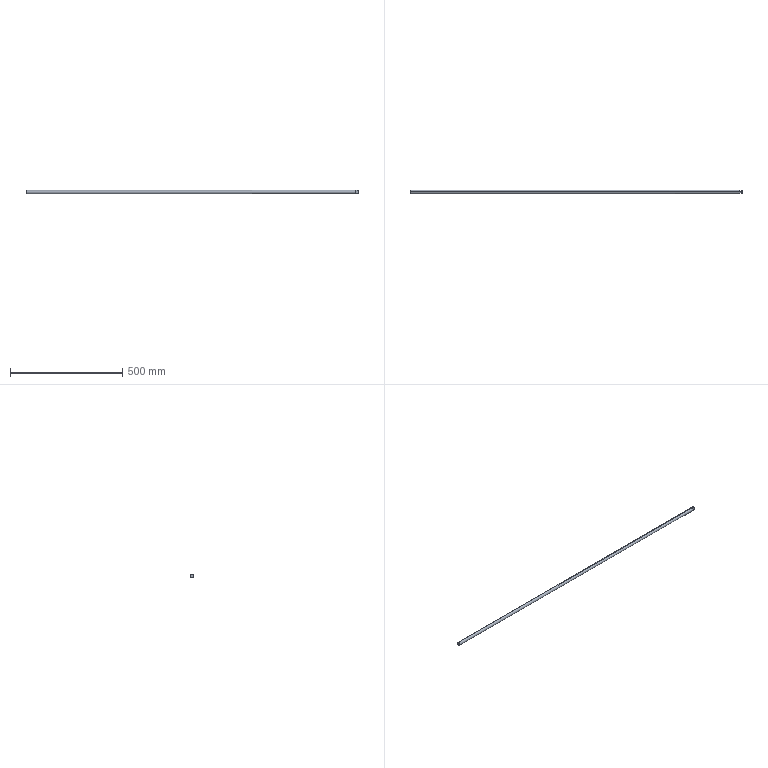Part | SolidWorks | features HoleWzd 2, Chamfer 1, Extrusion 1, ICE 1 | 1 solid | 13 faces | box 1480 x 15 x 15 mm | volume 261335 mm3 | plane 6 | cone 5 | cylinder 2 | commonest cylinder face diameters 15 x2
STEP:
#1=CARTESIAN_POINT('',(0.,0.,6.5));
#2=VERTEX_POINT('',#1);
#3=CARTESIAN_POINT('',(0.,0.,-6.5));
#4=VERTEX_POINT('',#3);
#5=CARTESIAN_POINT('',(0.,0.,0.));
#6=DIRECTION('',(-1.,0.,0.));
#7=DIRECTION('',(0.,0.,-1.));
#8=AXIS2_PLACEMENT_3D('',#5,#6,#7);
#9=CIRCLE('',#8,6.5);
#10=EDGE_CURVE('',#2,#4,#9,.T.);
#11=ORIENTED_EDGE('',*,*,#10,.F.);
#12=CARTESIAN_POINT('',(1.,0.,7.5));
#13=VERTEX_POINT('',#12);
#14=CARTESIAN_POINT('',(1.,0.,7.5));
#15=DIRECTION('',(0.7071,0.,0.7071));
#16=VECTOR('',#15,1000.);
#17=LINE('',#14,#16);
#18=EDGE_CURVE('',#2,#13,#17,.T.);
#19=ORIENTED_EDGE('',*,*,#18,.T.);
#20=CARTESIAN_POINT('',(1.,0.,-7.5));
#21=VERTEX_POINT('',#20);
#22=CARTESIAN_POINT('',(1.,0.,0.));
#23=DIRECTION('',(1.,0.,0.));
#24=DIRECTION('',(0.,0.,-1.));
#25=AXIS2_PLACEMENT_3D('',#22,#23,#24);
#26=CIRCLE('',#25,7.5);
#27=EDGE_CURVE('',#21,#13,#26,.T.);
#28=ORIENTED_EDGE('',*,*,#27,.F.);
#29=CARTESIAN_POINT('',(1.,0.,-7.5));
#30=DIRECTION('',(0.7071,0.,-0.7071));
#31=VECTOR('',#30,1000.);
#32=LINE('',#29,#31);
#33=EDGE_CURVE('',#4,#21,#32,.T.);
#34=ORIENTED_EDGE('',*,*,#33,.F.);
#35=EDGE_LOOP('',(#11,#19,#28,#34));
#36=FACE_OUTER_BOUND('',#35,.T.);
#37=CARTESIAN_POINT('',(1.,0.,0.));
#38=DIRECTION('',(1.,0.,0.));
#39=DIRECTION('',(0.,0.,-1.));
#40=AXIS2_PLACEMENT_3D('',#37,#38,#39);
#41=CONICAL_SURFACE('',#40,7.5,0.7854);
#42=ADVANCED_FACE('',(#36),#41,.T.);
#43=CARTESIAN_POINT('',(1479.,6.,-4.5));
#44=VERTEX_POINT('',#43);
#45=CARTESIAN_POINT('',(1479.,0.,-7.5));
#46=VERTEX_POINT('',#45);
#47=CARTESIAN_POINT('',(1479.,0.,0.));
#48=DIRECTION('',(-1.,0.,0.));
#49=DIRECTION('',(0.,0.,-1.));
#50=AXIS2_PLACEMENT_3D('',#47,#48,#49);
#51=CIRCLE('',#50,7.5);
#52=EDGE_CURVE('',#44,#46,#51,.T.);
#53=ORIENTED_EDGE('',*,*,#52,.T.);
#54=CARTESIAN_POINT('',(1480.,0.,-7.5));
#55=DIRECTION('',(-1.,0.,0.));
#56=VECTOR('',#55,1000.);
#57=LINE('',#54,#56);
#58=EDGE_CURVE('',#46,#21,#57,.T.);
#59=ORIENTED_EDGE('',*,*,#58,.T.);
#60=ORIENTED_EDGE('',*,*,#27,.T.);
#61=CARTESIAN_POINT('',(1479.,0.,7.5));
#62=VERTEX_POINT('',#61);
#63=CARTESIAN_POINT('',(1480.,0.,7.5));
#64=DIRECTION('',(-1.,0.,0.));
#65=VECTOR('',#64,1000.);
#66=LINE('',#63,#65);
#67=EDGE_CURVE('',#62,#13,#66,.T.);
#68=ORIENTED_EDGE('',*,*,#67,.F.);
#69=CARTESIAN_POINT('',(1479.,6.,4.5));
#70=VERTEX_POINT('',#69);
#71=CARTESIAN_POINT('',(1479.,0.,0.));
#72=DIRECTION('',(-1.,0.,0.));
#73=DIRECTION('',(0.,0.,-1.));
#74=AXIS2_PLACEMENT_3D('',#71,#72,#73);
#75=CIRCLE('',#74,7.5);
#76=EDGE_CURVE('',#62,#70,#75,.T.);
#77=ORIENTED_EDGE('',*,*,#76,.T.);
#78=CARTESIAN_POINT('',(1471.,6.,4.5));
#79=VERTEX_POINT('',#78);
#80=CARTESIAN_POINT('',(1480.,6.,4.5));
#81=DIRECTION('',(-1.,0.,0.));
#82=VECTOR('',#81,1000.);
#83=LINE('',#80,#82);
#84=EDGE_CURVE('',#70,#79,#83,.T.);
#85=ORIENTED_EDGE('',*,*,#84,.T.);
#86=CARTESIAN_POINT('',(1471.,6.,-4.5));
#87=VERTEX_POINT('',#86);
#88=CARTESIAN_POINT('',(1471.,0.,0.));
#89=DIRECTION('',(-1.,0.,0.));
#90=DIRECTION('',(0.,0.,1.));
#91=AXIS2_PLACEMENT_3D('',#88,#89,#90);
#92=CIRCLE('',#91,7.5);
#93=EDGE_CURVE('',#79,#87,#92,.T.);
#94=ORIENTED_EDGE('',*,*,#93,.T.);
#95=CARTESIAN_POINT('',(1480.,6.,-4.5));
#96=DIRECTION('',(1.,0.,0.));
#97=VECTOR('',#96,1000.);
#98=LINE('',#95,#97);
#99=EDGE_CURVE('',#87,#44,#98,.T.);
#100=ORIENTED_EDGE('',*,*,#99,.T.);
#101=EDGE_LOOP('',(#53,#59,#60,#68,#77,#85,#94,#100));
#102=FACE_OUTER_BOUND('',#101,.T.);
#103=CARTESIAN_POINT('',(1480.,0.,0.));
#104=DIRECTION('',(-1.,0.,0.));
#105=DIRECTION('',(0.,0.,1.));
#106=AXIS2_PLACEMENT_3D('',#103,#104,#105);
#107=CYLINDRICAL_SURFACE('',#106,7.5);
#108=ADVANCED_FACE('',(#102),#107,.T.);
#109=CARTESIAN_POINT('',(1480.,0.,6.5));
#110=VERTEX_POINT('',#109);
#111=CARTESIAN_POINT('',(1480.,-6.,2.5));
#112=VERTEX_POINT('',#111);
#113=CARTESIAN_POINT('',(1480.,0.,0.));
#114=DIRECTION('',(1.,0.,0.));
#115=DIRECTION('',(0.,0.,-1.));
#116=AXIS2_PLACEMENT_3D('',#113,#114,#115);
#117=CIRCLE('',#116,6.5);
#118=EDGE_CURVE('',#110,#112,#117,.T.);
#119=ORIENTED_EDGE('',*,*,#118,.F.);
#120=CARTESIAN_POINT('',(1480.,0.,6.5));
#121=DIRECTION('',(-0.7071,0.,0.7071));
#122=VECTOR('',#121,1000.);
#123=LINE('',#120,#122);
#124=EDGE_CURVE('',#110,#62,#123,.T.);
#125=ORIENTED_EDGE('',*,*,#124,.T.);
#126=CARTESIAN_POINT('',(1479.,-6.,4.5));
#127=VERTEX_POINT('',#126);
#128=CARTESIAN_POINT('',(1479.,0.,0.));
#129=DIRECTION('',(-1.,0.,0.));
#130=DIRECTION('',(0.,0.,-1.));
#131=AXIS2_PLACEMENT_3D('',#128,#129,#130);
#132=CIRCLE('',#131,7.5);
#133=EDGE_CURVE('',#127,#62,#132,.T.);
#134=ORIENTED_EDGE('',*,*,#133,.F.);
#135=CARTESIAN_POINT('',(1480.,-6.,2.5));
#136=CARTESIAN_POINT('',(1479.73,-6.,3.203));
#137=CARTESIAN_POINT('',(1479.383,-6.,3.862));
#138=CARTESIAN_POINT('',(1479.,-6.,4.5));
#139=B_SPLINE_CURVE_WITH_KNOTS('',3,(#135,#136,#137,#138),.UNSPECIFIED.,.F.,.F.,(4,4),(0.02153,0.02379),.UNSPECIFIED.);
#140=EDGE_CURVE('',#112,#127,#139,.T.);
#141=ORIENTED_EDGE('',*,*,#140,.F.);
#142=EDGE_LOOP('',(#119,#125,#134,#141));
#143=FACE_OUTER_BOUND('',#142,.T.);
#144=CARTESIAN_POINT('',(1480.,0.,0.));
#145=DIRECTION('',(-1.,0.,0.));
#146=DIRECTION('',(0.,0.,1.));
#147=AXIS2_PLACEMENT_3D('',#144,#145,#146);
#148=CONICAL_SURFACE('',#147,6.5,0.7854);
#149=ADVANCED_FACE('',(#143),#148,.T.);
#150=ORIENTED_EDGE('',*,*,#124,.F.);
#151=CARTESIAN_POINT('',(1480.,6.,2.5));
#152=VERTEX_POINT('',#151);
#153=CARTESIAN_POINT('',(1480.,0.,0.));
#154=DIRECTION('',(1.,0.,0.));
#155=DIRECTION('',(0.,0.,-1.));
#156=AXIS2_PLACEMENT_3D('',#153,#154,#155);
#157=CIRCLE('',#156,6.5);
#158=EDGE_CURVE('',#152,#110,#157,.T.);
#159=ORIENTED_EDGE('',*,*,#158,.F.);
#160=CARTESIAN_POINT('',(1479.,6.,4.5));
#161=CARTESIAN_POINT('',(1479.385,6.,3.859));
#162=CARTESIAN_POINT('',(1479.731,6.,3.198));
#163=CARTESIAN_POINT('',(1480.,6.,2.5));
#164=B_SPLINE_CURVE_WITH_KNOTS('',3,(#160,#161,#162,#163),.UNSPECIFIED.,.F.,.F.,(4,4),(0.01416,0.0164),.UNSPECIFIED.);
#165=EDGE_CURVE('',#70,#152,#164,.T.);
#166=ORIENTED_EDGE('',*,*,#165,.F.);
#167=ORIENTED_EDGE('',*,*,#76,.F.);
#168=EDGE_LOOP('',(#150,#159,#166,#167));
#169=FACE_OUTER_BOUND('',#168,.T.);
#170=CARTESIAN_POINT('',(1480.,0.,0.));
#171=DIRECTION('',(-1.,0.,0.));
#172=DIRECTION('',(0.,0.,1.));
#173=AXIS2_PLACEMENT_3D('',#170,#171,#172);
#174=CONICAL_SURFACE('',#173,6.5,0.7854);
#175=ADVANCED_FACE('',(#169),#174,.T.);
#176=ORIENTED_EDGE('',*,*,#58,.F.);
#177=CARTESIAN_POINT('',(1479.,-6.,-4.5));
#178=VERTEX_POINT('',#177);
#179=CARTESIAN_POINT('',(1479.,0.,0.));
#180=DIRECTION('',(-1.,0.,0.));
#181=DIRECTION('',(0.,0.,-1.));
#182=AXIS2_PLACEMENT_3D('',#179,#180,#181);
#183=CIRCLE('',#182,7.5);
#184=EDGE_CURVE('',#46,#178,#183,.T.);
#185=ORIENTED_EDGE('',*,*,#184,.T.);
#186=CARTESIAN_POINT('',(1471.,-6.,-4.5));
#187=VERTEX_POINT('',#186);
#188=CARTESIAN_POINT('',(1480.,-6.,-4.5));
#189=DIRECTION('',(-1.,0.,0.));
#190=VECTOR('',#189,1000.);
#191=LINE('',#188,#190);
#192=EDGE_CURVE('',#178,#187,#191,.T.);
#193=ORIENTED_EDGE('',*,*,#192,.T.);
#194=CARTESIAN_POINT('',(1471.,-6.,4.5));
#195=VERTEX_POINT('',#194);
#196=CARTESIAN_POINT('',(1471.,0.,0.));
#197=DIRECTION('',(-1.,0.,0.));
#198=DIRECTION('',(0.,0.,1.));
#199=AXIS2_PLACEMENT_3D('',#196,#197,#198);
#200=CIRCLE('',#199,7.5);
#201=EDGE_CURVE('',#187,#195,#200,.T.);
#202=ORIENTED_EDGE('',*,*,#201,.T.);
#203=CARTESIAN_POINT('',(1480.,-6.,4.5));
#204=DIRECTION('',(1.,0.,0.));
#205=VECTOR('',#204,1000.);
#206=LINE('',#203,#205);
#207=EDGE_CURVE('',#195,#127,#206,.T.);
#208=ORIENTED_EDGE('',*,*,#207,.T.);
#209=ORIENTED_EDGE('',*,*,#133,.T.);
#210=ORIENTED_EDGE('',*,*,#67,.T.);
#211=CARTESIAN_POINT('',(1.,0.,0.));
#212=DIRECTION('',(1.,0.,0.));
#213=DIRECTION('',(0.,0.,-1.));
#214=AXIS2_PLACEMENT_3D('',#211,#212,#213);
#215=CIRCLE('',#214,7.5);
#216=EDGE_CURVE('',#13,#21,#215,.T.);
#217=ORIENTED_EDGE('',*,*,#216,.T.);
#218=EDGE_LOOP('',(#176,#185,#193,#202,#208,#209,#210,#217));
#219=FACE_OUTER_BOUND('',#218,.T.);
#220=CARTESIAN_POINT('',(1480.,0.,0.));
#221=DIRECTION('',(-1.,0.,0.));
#222=DIRECTION('',(0.,0.,1.));
#223=AXIS2_PLACEMENT_3D('',#220,#221,#222);
#224=CYLINDRICAL_SURFACE('',#223,7.5);
#225=ADVANCED_FACE('',(#219),#224,.T.);
#226=CARTESIAN_POINT('',(1480.,6.,-2.5));
#227=VERTEX_POINT('',#226);
#228=CARTESIAN_POINT('',(1480.,6.,0.));
#229=DIRECTION('',(0.,0.,-1.));
#230=VECTOR('',#229,1000.);
#231=LINE('',#228,#230);
#232=EDGE_CURVE('',#152,#227,#231,.T.);
#233=ORIENTED_EDGE('',*,*,#232,.F.);
#234=ORIENTED_EDGE('',*,*,#158,.T.);
#235=ORIENTED_EDGE('',*,*,#118,.T.);
#236=CARTESIAN_POINT('',(1480.,-6.,-2.5));
#237=VERTEX_POINT('',#236);
#238=CARTESIAN_POINT('',(1480.,-6.,0.));
#239=DIRECTION('',(0.,0.,1.));
#240=VECTOR('',#239,1000.);
#241=LINE('',#238,#240);
#242=EDGE_CURVE('',#237,#112,#241,.T.);
#243=ORIENTED_EDGE('',*,*,#242,.F.);
#244=CARTESIAN_POINT('',(1480.,0.,0.));
#245=DIRECTION('',(1.,0.,0.));
#246=DIRECTION('',(0.,0.,-1.));
#247=AXIS2_PLACEMENT_3D('',#244,#245,#246);
#248=CIRCLE('',#247,6.5);
#249=EDGE_CURVE('',#237,#227,#248,.T.);
#250=ORIENTED_EDGE('',*,*,#249,.T.);
#251=EDGE_LOOP('',(#233,#234,#235,#243,#250));
#252=FACE_OUTER_BOUND('',#251,.T.);
#253=CARTESIAN_POINT('',(1480.,0.,0.));
#254=DIRECTION('',(1.,0.,0.));
#255=DIRECTION('',(0.,0.,-1.));
#256=AXIS2_PLACEMENT_3D('',#253,#254,#255);
#257=PLANE('',#256);
#258=ADVANCED_FACE('',(#252),#257,.T.);
#259=CARTESIAN_POINT('',(0.,0.,0.));
#260=DIRECTION('',(-1.,0.,0.));
#261=DIRECTION('',(0.,0.,-1.));
#262=AXIS2_PLACEMENT_3D('',#259,#260,#261);
#263=CIRCLE('',#262,6.5);
#264=EDGE_CURVE('',#4,#2,#263,.T.);
#265=ORIENTED_EDGE('',*,*,#264,.T.);
#266=ORIENTED_EDGE('',*,*,#10,.T.);
#267=EDGE_LOOP('',(#265,#266));
#268=FACE_OUTER_BOUND('',#267,.T.);
#269=CARTESIAN_POINT('',(0.,0.,0.));
#270=DIRECTION('',(1.,0.,0.));
#271=DIRECTION('',(0.,0.,-1.));
#272=AXIS2_PLACEMENT_3D('',#269,#270,#271);
#273=PLANE('',#272);
#274=ADVANCED_FACE('',(#268),#273,.F.);
#275=ORIENTED_EDGE('',*,*,#18,.F.);
#276=ORIENTED_EDGE('',*,*,#264,.F.);
#277=ORIENTED_EDGE('',*,*,#33,.T.);
#278=ORIENTED_EDGE('',*,*,#216,.F.);
#279=EDGE_LOOP('',(#275,#276,#277,#278));
#280=FACE_OUTER_BOUND('',#279,.T.);
#281=CARTESIAN_POINT('',(1.,0.,0.));
#282=DIRECTION('',(1.,0.,0.));
#283=DIRECTION('',(0.,0.,-1.));
#284=AXIS2_PLACEMENT_3D('',#281,#282,#283);
#285=CONICAL_SURFACE('',#284,7.5,0.7854);
#286=ADVANCED_FACE('',(#280),#285,.T.);
#287=CARTESIAN_POINT('',(1480.,6.,-2.5));
#288=CARTESIAN_POINT('',(1479.73,6.,-3.203));
#289=CARTESIAN_POINT('',(1479.383,6.,-3.862));
#290=CARTESIAN_POINT('',(1479.,6.,-4.5));
#291=B_SPLINE_CURVE_WITH_KNOTS('',3,(#287,#288,#289,#290),.UNSPECIFIED.,.F.,.F.,(4,4),(0.02153,0.02379),.UNSPECIFIED.);
#292=EDGE_CURVE('',#227,#44,#291,.T.);
#293=ORIENTED_EDGE('',*,*,#292,.F.);
#294=ORIENTED_EDGE('',*,*,#249,.F.);
#295=CARTESIAN_POINT('',(1479.,-6.,-4.5));
#296=CARTESIAN_POINT('',(1479.385,-6.,-3.859));
#297=CARTESIAN_POINT('',(1479.731,-6.,-3.198));
#298=CARTESIAN_POINT('',(1480.,-6.,-2.5));
#299=B_SPLINE_CURVE_WITH_KNOTS('',3,(#295,#296,#297,#298),.UNSPECIFIED.,.F.,.F.,(4,4),(0.01416,0.0164),.UNSPECIFIED.);
#300=EDGE_CURVE('',#178,#237,#299,.T.);
#301=ORIENTED_EDGE('',*,*,#300,.F.);
#302=ORIENTED_EDGE('',*,*,#184,.F.);
#303=ORIENTED_EDGE('',*,*,#52,.F.);
#304=EDGE_LOOP('',(#293,#294,#301,#302,#303));
#305=FACE_OUTER_BOUND('',#304,.T.);
#306=CARTESIAN_POINT('',(1480.,0.,0.));
#307=DIRECTION('',(-1.,0.,0.));
#308=DIRECTION('',(0.,0.,1.));
#309=AXIS2_PLACEMENT_3D('',#306,#307,#308);
#310=CONICAL_SURFACE('',#309,6.5,0.7854);
#311=ADVANCED_FACE('',(#305),#310,.T.);
#312=CARTESIAN_POINT('',(1471.,-6.,-7.5));
#313=DIRECTION('',(0.,0.,1.));
#314=VECTOR('',#313,1000.);
#315=LINE('',#312,#314);
#316=EDGE_CURVE('',#187,#195,#315,.T.);
#317=ORIENTED_EDGE('',*,*,#316,.T.);
#318=ORIENTED_EDGE('',*,*,#201,.F.);
#319=EDGE_LOOP('',(#317,#318));
#320=FACE_OUTER_BOUND('',#319,.T.);
#321=CARTESIAN_POINT('',(1471.,-7.9,-7.5));
#322=DIRECTION('',(-1.,0.,0.));
#323=DIRECTION('',(0.,0.,1.));
#324=AXIS2_PLACEMENT_3D('',#321,#322,#323);
#325=PLANE('',#324);
#326=ADVANCED_FACE('',(#320),#325,.F.);
#327=ORIENTED_EDGE('',*,*,#300,.T.);
#328=ORIENTED_EDGE('',*,*,#242,.T.);
#329=ORIENTED_EDGE('',*,*,#140,.T.);
#330=ORIENTED_EDGE('',*,*,#207,.F.);
#331=ORIENTED_EDGE('',*,*,#316,.F.);
#332=ORIENTED_EDGE('',*,*,#192,.F.);
#333=EDGE_LOOP('',(#327,#328,#329,#330,#331,#332));
#334=FACE_OUTER_BOUND('',#333,.T.);
#335=CARTESIAN_POINT('',(1514.567,-6.,-7.5));
#336=DIRECTION('',(0.,1.,0.));
#337=DIRECTION('',(-1.,0.,0.));
#338=AXIS2_PLACEMENT_3D('',#335,#336,#337);
#339=PLANE('',#338);
#340=ADVANCED_FACE('',(#334),#339,.F.);
#341=CARTESIAN_POINT('',(1471.,6.,-7.5));
#342=DIRECTION('',(0.,0.,1.));
#343=VECTOR('',#342,1000.);
#344=LINE('',#341,#343);
#345=EDGE_CURVE('',#87,#79,#344,.T.);
#346=ORIENTED_EDGE('',*,*,#345,.F.);
#347=ORIENTED_EDGE('',*,*,#93,.F.);
#348=EDGE_LOOP('',(#346,#347));
#349=FACE_OUTER_BOUND('',#348,.T.);
#350=CARTESIAN_POINT('',(1471.,7.9,-7.5));
#351=DIRECTION('',(-1.,0.,0.));
#352=DIRECTION('',(0.,0.,1.));
#353=AXIS2_PLACEMENT_3D('',#350,#351,#352);
#354=PLANE('',#353);
#355=ADVANCED_FACE('',(#349),#354,.F.);
#356=ORIENTED_EDGE('',*,*,#165,.T.);
#357=ORIENTED_EDGE('',*,*,#232,.T.);
#358=ORIENTED_EDGE('',*,*,#292,.T.);
#359=ORIENTED_EDGE('',*,*,#99,.F.);
#360=ORIENTED_EDGE('',*,*,#345,.T.);
#361=ORIENTED_EDGE('',*,*,#84,.F.);
#362=EDGE_LOOP('',(#356,#357,#358,#359,#360,#361));
#363=FACE_OUTER_BOUND('',#362,.T.);
#364=CARTESIAN_POINT('',(1514.567,6.,-7.5));
#365=DIRECTION('',(0.,-1.,0.));
#366=DIRECTION('',(1.,0.,0.));
#367=AXIS2_PLACEMENT_3D('',#364,#365,#366);
#368=PLANE('',#367);
#369=ADVANCED_FACE('',(#363),#368,.F.);
#370=CLOSED_SHELL('',(#42,#108,#149,#175,#225,#258,#274,#286,#311,#326,#340,#355,#369));
#371=MANIFOLD_SOLID_BREP('',#370);
#372=CARTESIAN_POINT('',(0.,0.,0.));
#373=DIRECTION('',(0.,0.,1.));
#374=DIRECTION('',(1.,0.,0.));
#375=AXIS2_PLACEMENT_3D('',#372,#373,#374);
#376=(LENGTH_UNIT()NAMED_UNIT(*)SI_UNIT(.MILLI.,.METRE.));
#377=UNCERTAINTY_MEASURE_WITH_UNIT(LENGTH_MEASURE(0.00001),#376,'','');
#378=(NAMED_UNIT(*)PLANE_ANGLE_UNIT()SI_UNIT($,.RADIAN.));
#379=(NAMED_UNIT(*)SI_UNIT($,.STERADIAN.)SOLID_ANGLE_UNIT());
#380=(GEOMETRIC_REPRESENTATION_CONTEXT(3)GLOBAL_UNCERTAINTY_ASSIGNED_CONTEXT((#377))GLOBAL_UNIT_ASSIGNED_CONTEXT((#376,#378,#379))REPRESENTATION_CONTEXT('',''));
#381=ADVANCED_BREP_SHAPE_REPRESENTATION('',(#371,#375),#380);